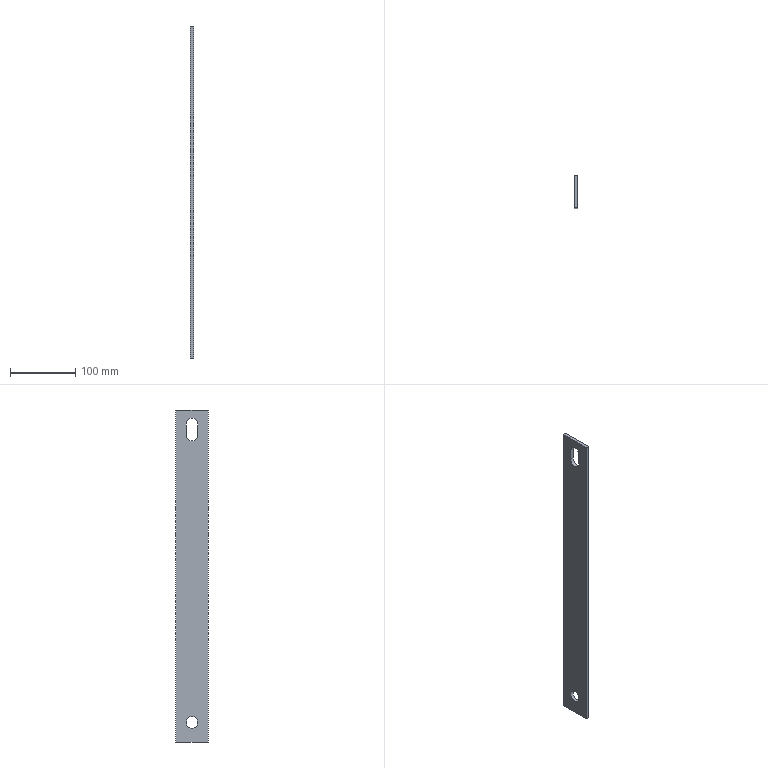Part | NX | features MAIN_BODY 2 | 1 solid | 11 faces | box 5 x 50 x 510 mm | volume 123425 mm3 | plane 8 | cylinder 3 | commonest cylinder face diameters 18 x3
STEP:
#1=CARTESIAN_POINT('',(2255.,294.,288.5));
#2=VERTEX_POINT('',#1);
#3=CARTESIAN_POINT('',(2255.,276.,288.5));
#4=VERTEX_POINT('',#3);
#5=CARTESIAN_POINT('',(2255.,285.,288.5));
#6=DIRECTION('',(1.,0.,0.));
#7=DIRECTION('',(0.,1.,0.));
#8=AXIS2_PLACEMENT_3D('',#5,#6,#7);
#9=CIRCLE('',#8,9.);
#10=EDGE_CURVE('',#2,#4,#9,.T.);
#11=ORIENTED_EDGE('',*,*,#10,.F.);
#12=CARTESIAN_POINT('',(2260.,294.,288.5));
#13=VERTEX_POINT('',#12);
#14=CARTESIAN_POINT('',(2260.,294.,288.5));
#15=DIRECTION('',(-1.,0.,0.));
#16=VECTOR('',#15,1000.);
#17=LINE('',#14,#16);
#18=EDGE_CURVE('',#13,#2,#17,.T.);
#19=ORIENTED_EDGE('',*,*,#18,.F.);
#20=CARTESIAN_POINT('',(2260.,276.,288.5));
#21=VERTEX_POINT('',#20);
#22=CARTESIAN_POINT('',(2260.,285.,288.5));
#23=DIRECTION('',(1.,0.,0.));
#24=DIRECTION('',(0.,1.,0.));
#25=AXIS2_PLACEMENT_3D('',#22,#23,#24);
#26=CIRCLE('',#25,9.);
#27=EDGE_CURVE('',#13,#21,#26,.T.);
#28=ORIENTED_EDGE('',*,*,#27,.T.);
#29=CARTESIAN_POINT('',(2260.,276.,288.5));
#30=DIRECTION('',(-1.,0.,0.));
#31=VECTOR('',#30,1000.);
#32=LINE('',#29,#31);
#33=EDGE_CURVE('',#21,#4,#32,.T.);
#34=ORIENTED_EDGE('',*,*,#33,.T.);
#35=EDGE_LOOP('',(#11,#19,#28,#34));
#36=FACE_BOUND('',#35,.T.);
#37=CARTESIAN_POINT('',(2260.,285.,288.5));
#38=DIRECTION('',(-1.,0.,0.));
#39=DIRECTION('',(0.,1.,0.));
#40=AXIS2_PLACEMENT_3D('',#37,#38,#39);
#41=CYLINDRICAL_SURFACE('',#40,9.);
#42=ADVANCED_FACE('',(#36),#41,.F.);
#43=CARTESIAN_POINT('',(2255.,294.,271.5));
#44=VERTEX_POINT('',#43);
#45=CARTESIAN_POINT('',(2255.,294.,288.5));
#46=DIRECTION('',(0.,0.,-1.));
#47=VECTOR('',#46,1000.);
#48=LINE('',#45,#47);
#49=EDGE_CURVE('',#2,#44,#48,.T.);
#50=ORIENTED_EDGE('',*,*,#49,.T.);
#51=CARTESIAN_POINT('',(2260.,294.,271.5));
#52=VERTEX_POINT('',#51);
#53=CARTESIAN_POINT('',(2260.,294.,271.5));
#54=DIRECTION('',(-1.,0.,0.));
#55=VECTOR('',#54,1000.);
#56=LINE('',#53,#55);
#57=EDGE_CURVE('',#52,#44,#56,.T.);
#58=ORIENTED_EDGE('',*,*,#57,.F.);
#59=CARTESIAN_POINT('',(2260.,294.,288.5));
#60=DIRECTION('',(0.,0.,-1.));
#61=VECTOR('',#60,1000.);
#62=LINE('',#59,#61);
#63=EDGE_CURVE('',#13,#52,#62,.T.);
#64=ORIENTED_EDGE('',*,*,#63,.F.);
#65=ORIENTED_EDGE('',*,*,#18,.T.);
#66=EDGE_LOOP('',(#50,#58,#64,#65));
#67=FACE_BOUND('',#66,.T.);
#68=CARTESIAN_POINT('',(2260.,294.,288.5));
#69=DIRECTION('',(0.,-1.,0.));
#70=DIRECTION('',(-1.,0.,0.));
#71=AXIS2_PLACEMENT_3D('',#68,#69,#70);
#72=PLANE('',#71);
#73=ADVANCED_FACE('',(#67),#72,.T.);
#74=CARTESIAN_POINT('',(2255.,276.,271.5));
#75=VERTEX_POINT('',#74);
#76=CARTESIAN_POINT('',(2255.,285.,271.5));
#77=DIRECTION('',(1.,0.,0.));
#78=DIRECTION('',(0.,1.,0.));
#79=AXIS2_PLACEMENT_3D('',#76,#77,#78);
#80=CIRCLE('',#79,9.);
#81=EDGE_CURVE('',#75,#44,#80,.T.);
#82=ORIENTED_EDGE('',*,*,#81,.F.);
#83=CARTESIAN_POINT('',(2260.,276.,271.5));
#84=VERTEX_POINT('',#83);
#85=CARTESIAN_POINT('',(2260.,276.,271.5));
#86=DIRECTION('',(-1.,0.,0.));
#87=VECTOR('',#86,1000.);
#88=LINE('',#85,#87);
#89=EDGE_CURVE('',#84,#75,#88,.T.);
#90=ORIENTED_EDGE('',*,*,#89,.F.);
#91=CARTESIAN_POINT('',(2260.,285.,271.5));
#92=DIRECTION('',(1.,0.,0.));
#93=DIRECTION('',(0.,1.,0.));
#94=AXIS2_PLACEMENT_3D('',#91,#92,#93);
#95=CIRCLE('',#94,9.);
#96=EDGE_CURVE('',#84,#52,#95,.T.);
#97=ORIENTED_EDGE('',*,*,#96,.T.);
#98=ORIENTED_EDGE('',*,*,#57,.T.);
#99=EDGE_LOOP('',(#82,#90,#97,#98));
#100=FACE_BOUND('',#99,.T.);
#101=CARTESIAN_POINT('',(2260.,285.,271.5));
#102=DIRECTION('',(-1.,0.,0.));
#103=DIRECTION('',(0.,1.,0.));
#104=AXIS2_PLACEMENT_3D('',#101,#102,#103);
#105=CYLINDRICAL_SURFACE('',#104,9.);
#106=ADVANCED_FACE('',(#100),#105,.F.);
#107=CARTESIAN_POINT('',(2255.,310.,-200.));
#108=VERTEX_POINT('',#107);
#109=CARTESIAN_POINT('',(2255.,310.,310.));
#110=VERTEX_POINT('',#109);
#111=CARTESIAN_POINT('',(2255.,310.,-200.));
#112=DIRECTION('',(0.,0.,1.));
#113=VECTOR('',#112,1000.);
#114=LINE('',#111,#113);
#115=EDGE_CURVE('',#108,#110,#114,.T.);
#116=ORIENTED_EDGE('',*,*,#115,.T.);
#117=CARTESIAN_POINT('',(2260.,310.,310.));
#118=VERTEX_POINT('',#117);
#119=CARTESIAN_POINT('',(2260.,310.,310.));
#120=DIRECTION('',(-1.,0.,0.));
#121=VECTOR('',#120,1000.);
#122=LINE('',#119,#121);
#123=EDGE_CURVE('',#118,#110,#122,.T.);
#124=ORIENTED_EDGE('',*,*,#123,.F.);
#125=CARTESIAN_POINT('',(2260.,310.,-200.));
#126=VERTEX_POINT('',#125);
#127=CARTESIAN_POINT('',(2260.,310.,-200.));
#128=DIRECTION('',(0.,0.,1.));
#129=VECTOR('',#128,1000.);
#130=LINE('',#127,#129);
#131=EDGE_CURVE('',#126,#118,#130,.T.);
#132=ORIENTED_EDGE('',*,*,#131,.F.);
#133=CARTESIAN_POINT('',(2260.,310.,-200.));
#134=DIRECTION('',(-1.,0.,0.));
#135=VECTOR('',#134,1000.);
#136=LINE('',#133,#135);
#137=EDGE_CURVE('',#126,#108,#136,.T.);
#138=ORIENTED_EDGE('',*,*,#137,.T.);
#139=EDGE_LOOP('',(#116,#124,#132,#138));
#140=FACE_BOUND('',#139,.T.);
#141=CARTESIAN_POINT('',(2260.,310.,-200.));
#142=DIRECTION('',(0.,1.,0.));
#143=DIRECTION('',(0.,0.,1.));
#144=AXIS2_PLACEMENT_3D('',#141,#142,#143);
#145=PLANE('',#144);
#146=ADVANCED_FACE('',(#140),#145,.T.);
#147=CARTESIAN_POINT('',(2255.,260.,310.));
#148=VERTEX_POINT('',#147);
#149=CARTESIAN_POINT('',(2255.,310.,310.));
#150=DIRECTION('',(0.,-1.,0.));
#151=VECTOR('',#150,1000.);
#152=LINE('',#149,#151);
#153=EDGE_CURVE('',#110,#148,#152,.T.);
#154=ORIENTED_EDGE('',*,*,#153,.T.);
#155=CARTESIAN_POINT('',(2260.,260.,310.));
#156=VERTEX_POINT('',#155);
#157=CARTESIAN_POINT('',(2260.,260.,310.));
#158=DIRECTION('',(-1.,0.,0.));
#159=VECTOR('',#158,1000.);
#160=LINE('',#157,#159);
#161=EDGE_CURVE('',#156,#148,#160,.T.);
#162=ORIENTED_EDGE('',*,*,#161,.F.);
#163=CARTESIAN_POINT('',(2260.,310.,310.));
#164=DIRECTION('',(0.,-1.,0.));
#165=VECTOR('',#164,1000.);
#166=LINE('',#163,#165);
#167=EDGE_CURVE('',#118,#156,#166,.T.);
#168=ORIENTED_EDGE('',*,*,#167,.F.);
#169=ORIENTED_EDGE('',*,*,#123,.T.);
#170=EDGE_LOOP('',(#154,#162,#168,#169));
#171=FACE_BOUND('',#170,.T.);
#172=CARTESIAN_POINT('',(2260.,310.,310.));
#173=DIRECTION('',(0.,0.,1.));
#174=DIRECTION('',(-1.,0.,0.));
#175=AXIS2_PLACEMENT_3D('',#172,#173,#174);
#176=PLANE('',#175);
#177=ADVANCED_FACE('',(#171),#176,.T.);
#178=CARTESIAN_POINT('',(2255.,260.,-200.));
#179=VERTEX_POINT('',#178);
#180=CARTESIAN_POINT('',(2255.,260.,310.));
#181=DIRECTION('',(0.,0.,-1.));
#182=VECTOR('',#181,1000.);
#183=LINE('',#180,#182);
#184=EDGE_CURVE('',#148,#179,#183,.T.);
#185=ORIENTED_EDGE('',*,*,#184,.T.);
#186=CARTESIAN_POINT('',(2260.,260.,-200.));
#187=VERTEX_POINT('',#186);
#188=CARTESIAN_POINT('',(2260.,260.,-200.));
#189=DIRECTION('',(-1.,0.,0.));
#190=VECTOR('',#189,1000.);
#191=LINE('',#188,#190);
#192=EDGE_CURVE('',#187,#179,#191,.T.);
#193=ORIENTED_EDGE('',*,*,#192,.F.);
#194=CARTESIAN_POINT('',(2260.,260.,310.));
#195=DIRECTION('',(0.,0.,-1.));
#196=VECTOR('',#195,1000.);
#197=LINE('',#194,#196);
#198=EDGE_CURVE('',#156,#187,#197,.T.);
#199=ORIENTED_EDGE('',*,*,#198,.F.);
#200=ORIENTED_EDGE('',*,*,#161,.T.);
#201=EDGE_LOOP('',(#185,#193,#199,#200));
#202=FACE_BOUND('',#201,.T.);
#203=CARTESIAN_POINT('',(2260.,260.,310.));
#204=DIRECTION('',(0.,-1.,0.));
#205=DIRECTION('',(0.,0.,-1.));
#206=AXIS2_PLACEMENT_3D('',#203,#204,#205);
#207=PLANE('',#206);
#208=ADVANCED_FACE('',(#202),#207,.T.);
#209=CARTESIAN_POINT('',(2260.,294.,-170.));
#210=VERTEX_POINT('',#209);
#211=CARTESIAN_POINT('',(2260.,285.,-170.));
#212=DIRECTION('',(1.,0.,0.));
#213=DIRECTION('',(0.,1.,0.));
#214=AXIS2_PLACEMENT_3D('',#211,#212,#213);
#215=CIRCLE('',#214,9.);
#216=EDGE_CURVE('',#210,#210,#215,.T.);
#217=ORIENTED_EDGE('',*,*,#216,.T.);
#218=EDGE_LOOP('',(#217));
#219=FACE_BOUND('',#218,.T.);
#220=CARTESIAN_POINT('',(2255.,294.,-170.));
#221=VERTEX_POINT('',#220);
#222=CARTESIAN_POINT('',(2255.,285.,-170.));
#223=DIRECTION('',(1.,0.,0.));
#224=DIRECTION('',(0.,1.,0.));
#225=AXIS2_PLACEMENT_3D('',#222,#223,#224);
#226=CIRCLE('',#225,9.);
#227=EDGE_CURVE('',#221,#221,#226,.T.);
#228=ORIENTED_EDGE('',*,*,#227,.F.);
#229=EDGE_LOOP('',(#228));
#230=FACE_BOUND('',#229,.T.);
#231=CARTESIAN_POINT('',(2260.,285.,-170.));
#232=DIRECTION('',(-1.,0.,0.));
#233=DIRECTION('',(0.,1.,0.));
#234=AXIS2_PLACEMENT_3D('',#231,#232,#233);
#235=CYLINDRICAL_SURFACE('',#234,9.);
#236=ADVANCED_FACE('',(#219,#230),#235,.F.);
#237=CARTESIAN_POINT('',(2255.,260.,-200.));
#238=DIRECTION('',(0.,1.,0.));
#239=VECTOR('',#238,1000.);
#240=LINE('',#237,#239);
#241=EDGE_CURVE('',#179,#108,#240,.T.);
#242=ORIENTED_EDGE('',*,*,#241,.T.);
#243=ORIENTED_EDGE('',*,*,#137,.F.);
#244=CARTESIAN_POINT('',(2260.,260.,-200.));
#245=DIRECTION('',(0.,1.,0.));
#246=VECTOR('',#245,1000.);
#247=LINE('',#244,#246);
#248=EDGE_CURVE('',#187,#126,#247,.T.);
#249=ORIENTED_EDGE('',*,*,#248,.F.);
#250=ORIENTED_EDGE('',*,*,#192,.T.);
#251=EDGE_LOOP('',(#242,#243,#249,#250));
#252=FACE_BOUND('',#251,.T.);
#253=CARTESIAN_POINT('',(2260.,260.,-200.));
#254=DIRECTION('',(0.,0.,-1.));
#255=DIRECTION('',(1.,0.,0.));
#256=AXIS2_PLACEMENT_3D('',#253,#254,#255);
#257=PLANE('',#256);
#258=ADVANCED_FACE('',(#252),#257,.T.);
#259=CARTESIAN_POINT('',(2255.,276.,271.5));
#260=DIRECTION('',(0.,0.,1.));
#261=VECTOR('',#260,1000.);
#262=LINE('',#259,#261);
#263=EDGE_CURVE('',#75,#4,#262,.T.);
#264=ORIENTED_EDGE('',*,*,#263,.T.);
#265=ORIENTED_EDGE('',*,*,#33,.F.);
#266=CARTESIAN_POINT('',(2260.,276.,271.5));
#267=DIRECTION('',(0.,0.,1.));
#268=VECTOR('',#267,1000.);
#269=LINE('',#266,#268);
#270=EDGE_CURVE('',#84,#21,#269,.T.);
#271=ORIENTED_EDGE('',*,*,#270,.F.);
#272=ORIENTED_EDGE('',*,*,#89,.T.);
#273=EDGE_LOOP('',(#264,#265,#271,#272));
#274=FACE_BOUND('',#273,.T.);
#275=CARTESIAN_POINT('',(2260.,276.,271.5));
#276=DIRECTION('',(0.,1.,0.));
#277=DIRECTION('',(1.,0.,0.));
#278=AXIS2_PLACEMENT_3D('',#275,#276,#277);
#279=PLANE('',#278);
#280=ADVANCED_FACE('',(#274),#279,.T.);
#281=ORIENTED_EDGE('',*,*,#131,.T.);
#282=ORIENTED_EDGE('',*,*,#167,.T.);
#283=ORIENTED_EDGE('',*,*,#198,.T.);
#284=ORIENTED_EDGE('',*,*,#248,.T.);
#285=EDGE_LOOP('',(#281,#282,#283,#284));
#286=FACE_BOUND('',#285,.T.);
#287=ORIENTED_EDGE('',*,*,#216,.F.);
#288=EDGE_LOOP('',(#287));
#289=FACE_BOUND('',#288,.T.);
#290=ORIENTED_EDGE('',*,*,#27,.F.);
#291=ORIENTED_EDGE('',*,*,#63,.T.);
#292=ORIENTED_EDGE('',*,*,#96,.F.);
#293=ORIENTED_EDGE('',*,*,#270,.T.);
#294=EDGE_LOOP('',(#290,#291,#292,#293));
#295=FACE_BOUND('',#294,.T.);
#296=CARTESIAN_POINT('',(2260.,310.,310.));
#297=DIRECTION('',(-1.,0.,0.));
#298=DIRECTION('',(0.,1.,0.));
#299=AXIS2_PLACEMENT_3D('',#296,#297,#298);
#300=PLANE('',#299);
#301=ADVANCED_FACE('',(#286,#289,#295),#300,.F.);
#302=ORIENTED_EDGE('',*,*,#115,.F.);
#303=ORIENTED_EDGE('',*,*,#241,.F.);
#304=ORIENTED_EDGE('',*,*,#184,.F.);
#305=ORIENTED_EDGE('',*,*,#153,.F.);
#306=EDGE_LOOP('',(#302,#303,#304,#305));
#307=FACE_BOUND('',#306,.T.);
#308=ORIENTED_EDGE('',*,*,#227,.T.);
#309=EDGE_LOOP('',(#308));
#310=FACE_BOUND('',#309,.T.);
#311=ORIENTED_EDGE('',*,*,#10,.T.);
#312=ORIENTED_EDGE('',*,*,#263,.F.);
#313=ORIENTED_EDGE('',*,*,#81,.T.);
#314=ORIENTED_EDGE('',*,*,#49,.F.);
#315=EDGE_LOOP('',(#311,#312,#313,#314));
#316=FACE_BOUND('',#315,.T.);
#317=CARTESIAN_POINT('',(2255.,310.,310.));
#318=DIRECTION('',(-1.,0.,0.));
#319=DIRECTION('',(0.,1.,0.));
#320=AXIS2_PLACEMENT_3D('',#317,#318,#319);
#321=PLANE('',#320);
#322=ADVANCED_FACE('',(#307,#310,#316),#321,.T.);
#323=CLOSED_SHELL('',(#42,#73,#106,#146,#177,#208,#236,#258,#280,#301,#322));
#324=MANIFOLD_SOLID_BREP('',#323);
#325=(LENGTH_UNIT()NAMED_UNIT(*)SI_UNIT(.MILLI.,.METRE.));
#326=UNCERTAINTY_MEASURE_WITH_UNIT(LENGTH_MEASURE(0.00001),#325,'','');
#327=(NAMED_UNIT(*)PLANE_ANGLE_UNIT()SI_UNIT($,.RADIAN.));
#328=(NAMED_UNIT(*)SI_UNIT($,.STERADIAN.)SOLID_ANGLE_UNIT());
#329=(GEOMETRIC_REPRESENTATION_CONTEXT(3)GLOBAL_UNCERTAINTY_ASSIGNED_CONTEXT((#326))GLOBAL_UNIT_ASSIGNED_CONTEXT((#325,#327,#328))REPRESENTATION_CONTEXT('',''));
#330=ADVANCED_BREP_SHAPE_REPRESENTATION('',(#324),#329);